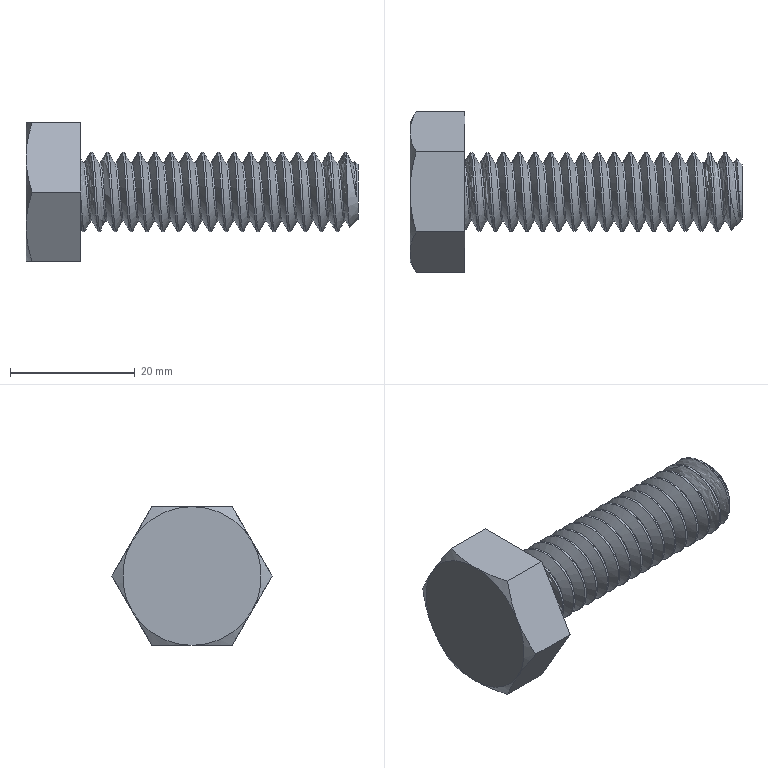Part | SolidWorks | features ICE 2, Chamfer 1, Extrusion 1, Helix 1, Revolution 1, Scale 1, SweepCut 1 | 1 solid | 55 faces | box 53.181 x 25.663 x 22.225 mm | volume 8007 mm3 | cylinder 35 | plane 9 | cone 8 | spline 3 | commonest cylinder face diameters 12.7 x35